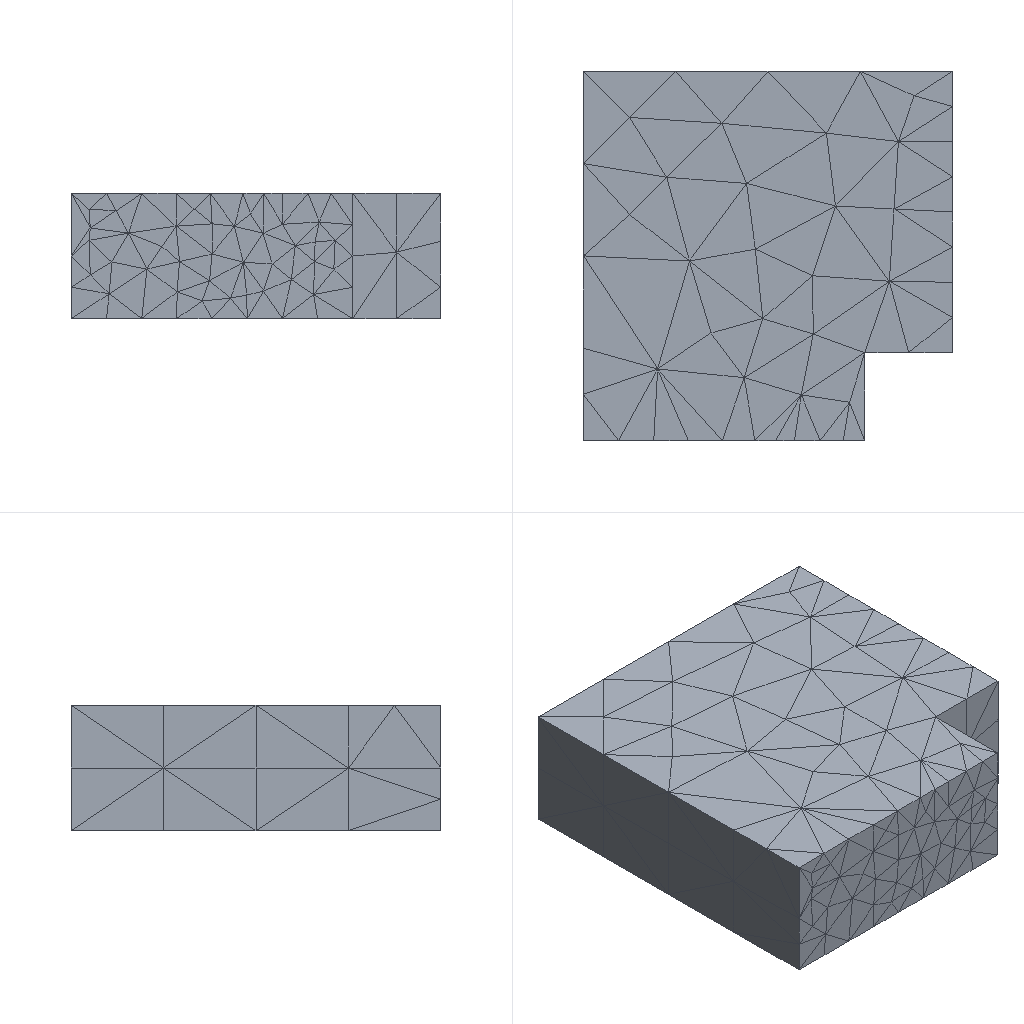Simulation study | ansys electronics desktop
Set-up summary:
category,name,step,type,value,unit,region
solver,ansys_electronics_desktop
units,length mm,,stated,model units
analysis,DESIGN_1,,HFSS Modal Network,design_type=HFSS
setup,Setup1,DESIGN_1,HfssDriven,frequency=10GHz; max_passes=6; max_delta_s=0.02
sweep,Sweep1,Setup1,Discrete,8GHz..12GHz n=9 step=
mesh,nodes,,,n/a (no mesh stored)
mesh,elements,,,n/a (no mesh stored)
material,vacuum,,permittivity,1
load,1,DESIGN_1,wave port,,,faces 9
load,2,DESIGN_1,wave port,,,faces 40
bc,PerfE,DESIGN_1,perfect e,,,"faces 7, 10, 11, 8, 12, 37"
Ansys Electronics Desktop project file, long lists of numbers shortened, first 464 of 1677 lines:
$begin 'AnsoftProject'
	Created='Fri Sep  4 17:11:43 2026'
	Product='ElectronicsDesktop'
	FileOwnedByWorkbench=false
	$begin 'Desktop'
		Version(2026, 1)
		InfrastructureVersion(1, 0)
		$begin 'FactoryHeader'
			$begin 'geometry3deditor'
				KernelVersion(2, 0)
				ProjectContainsGeometry3D='1'
			$end 'geometry3deditor'
		$end 'FactoryHeader'
	$end 'Desktop'
	UsesAdvancedFeatures=false
	PreviewImageDesignId=1
	NextUniqueID=0
	MoveBackwards=false
	$begin 'HFSSEnvironment'
		Version(1, 0)
	$end 'HFSSEnvironment'
	$begin 'PlanarEMEnvironment'
		Version(1, 0)
	$end 'PlanarEMEnvironment'
	$begin 'Q3DEnvironment'
		Version(1, 0)
	$end 'Q3DEnvironment'
	$begin '2DExtractorEnvironment'
		Version(1, 0)
	$end '2DExtractorEnvironment'
	$begin 'NexximEnvironment'
		Version(1, 0)
	$end 'NexximEnvironment'
	$begin 'NexximNetlistEnvironment'
		Version(1, 0)
	$end 'NexximNetlistEnvironment'
	$begin 'EmitEnvironment'
		Version(1, 0)
	$end 'EmitEnvironment'
	$begin 'Maxwell3DEnvironment'
		Version(1, 0)
	$end 'Maxwell3DEnvironment'
	$begin 'Maxwell2DEnvironment'
		Version(1, 0)
	$end 'Maxwell2DEnvironment'
	$begin 'RMxprtEnvironment'
		Version(1, 0)
	$end 'RMxprtEnvironment'
	$begin 'MaxCirEnvironment'
		Version(1, 0)
	$end 'MaxCirEnvironment'
	$begin 'SimplorerEnvironment'
		Version(1, 0)
	$end 'SimplorerEnvironment'
	$begin 'IcepakEnvironment'
		Version(1, 0)
	$end 'IcepakEnvironment'
	$begin 'IcepakFEAEnvironment'
		Version(1, 0)
	$end 'IcepakFEAEnvironment'
	$begin 'SchematicEnvironment'
		Version(1, 0)
	$end 'SchematicEnvironment'
	$begin 'geometry3deditor'
		Version(1, 0)
	$end 'geometry3deditor'
	ReadVersion=12
	$begin 'DesignMgrEnvironment'
		CompInstCounter=1
		GPortCounter=0
		NetCounter=0
		Alias('Ieee;Simplorer Elements\\Ieee', 'Std;Simplorer Elements\\Std', 'Basic_VHDLAMS;Simplorer Elements\\Basic Elements VHDLAMS\\Basic Elements VHDLAMS', 'Digital_Elements;Simplorer Elements\\Digital Elements\\Digital Elements', 'Transformations;Simplorer Elements\\Tools\\Transformations\\Transformations', 'HEV_VHDLAMS;Simplorer Elements\\HEV VHDLAMS\\HEV VHDLAMS', 'automotive_vda;Simplorer Elem
	$end 'DesignMgrEnvironment'
	$begin 'ProjectDatasets'
		NextUniqueID=0
		MoveBackwards=false
		DatasetType='ProjectDatasetType'
		$begin 'DatasetDefinitions'
		$end 'DatasetDefinitions'
	$end 'ProjectDatasets'
	VariableOrders[0:]
	$begin 'Definitions'
		$begin 'Materials'
			$begin 'vacuum'
				CoordinateSystemType='Cartesian'
				BulkOrSurfaceType=1
				$begin 'PhysicsTypes'
					set('Electromagnetic')
				$end 'PhysicsTypes'
				$begin 'AttachedData'
					$begin 'MatAppearanceData'
						property_data='appearance_data'
						Red=230
						Green=230
						Blue=230
						Transparency=0.95
					$end 'MatAppearanceData'
				$end 'AttachedData'
				permittivity='1'
				ModTime=1499970477
				Library='Materials'
				LibLocation='SysLibrary'
				ModSinceLib=false
			$end 'vacuum'
		$end 'Materials'
		$begin 'SurfaceMaterials'
			$begin 'Steel-oxidised-surface'
				CoordinateSystemType='Cartesian'
				BulkOrSurfaceType=2
				$begin 'PhysicsTypes'
					set('Thermal')
				$end 'PhysicsTypes'
				surface_emissivity='0.8'
				ModTime=1461288057
				Library='SurfaceMaterials'
				LibLocation='SysLibrary'
				ModSinceLib=false
			$end 'Steel-oxidised-surface'
		$end 'SurfaceMaterials'
		$begin 'Scripts'
		$end 'Scripts'
		$begin 'AnsysComponents'
			NextUniqueID=0
			MoveBackwards=false
			$begin 'AnsysComponentDefinitions'
			$end 'AnsysComponentDefinitions'
		$end 'AnsysComponents'
		$begin 'Symbols'
			$begin 'DESIGN_1'
				ModTime=1788513103
				Library=''
				ModSinceLib=false
				LibLocation='Project'
				HighestLevel=1
				Normalize=true
				InitialLevels(0, 1)
				$begin 'Graphics'
					Rect(0, 0, 0, 0, 0.00254, 0.00254, 0.00508, 0.00508, 0, 0, 0)
					Rect(0, 1, 0, 0, 0.0004233, 0.00254, 0.0004233, 0.0004233, 0, 0, 0)
				$end 'Graphics'
			$end 'DESIGN_1'
		$end 'Symbols'
		$begin 'DefInfo'
			DESIGN_1(1002, 0, 0, 0, '', 1788513103, '', 'DESIGN_1', '', '', '', '', '', 'Design.bmp', '', 'Project', '', '', 1788513103, '', 0, 0)
		$end 'DefInfo'
		$begin 'Compdefs'
			$begin 'DESIGN_1'
				Library=''
				CircuitEnv=0
				Refbase='U'
				NumParts=1
				ModSinceLib=true
				$begin 'Properties'
					TextProp('Representation', 'SRD', '', 'DESIGN_1')
					TextProp('Owner', 'SRD', '', 'HFSS')
				$end 'Properties'
				CompExtID=6
				$begin 'Parameters'
					ButtonProp('CosimDefinition', 'D', '', 'Edit', 'Edit', 40501, ButtonPropClientData())
					MenuProp('CoSimulator', 'D', '', 'DefaultNetlist', 0)
				$end 'Parameters'
				$begin 'CosimDefinitions'
					$begin 'CosimDefinition'
						CosimulatorType=4
						CosimDefName='DefaultNetlist'
						IsDefinition=true
						Connect=true
						Data()
						GRef()
					$end 'CosimDefinition'
					DefaultCosim='DefaultNetlist'
				$end 'CosimDefinitions'
			$end 'DESIGN_1'
		$end 'Compdefs'
	$end 'Definitions'
	DesignIDServer=2
	MoveBackwards=false
	$begin 'HFSSModel'
		RepRewriteV2=true
		Name='DESIGN_1'
		DesignID=0
		'Use Advanced DC Extrapolation'=false
		'Use Power S'=false
		'Export FRTM After Simulation'=false
		'Export Rays After Simulation'=false
		'Export After Simulation'=false
		'Allow Material Override'=false
		'Calculate Lossy Dielectrics'=false
		'Perform Minimal validation'=false
		$begin 'TemperatureSettings'
			IncludeTemperatureDependence=false
			EnableFeedback=false
			Temperatures(6, '22cel')
		$end 'TemperatureSettings'
		ObjsEnabledForDeformation()
		'Port Validation Settings'='Standard'
		'Save Adaptive support files'=false
		SolutionType='HFSS Modal Network'
		$begin 'DrivenOptions'
			AutoOpen=false
		$end 'DrivenOptions'
		HasTransientSetups=false
		MaterialDensity=1
		MassOfTissue=1
		VoxelSize=1
		TissueObjectList=-1
		AverageSarMethod=0
		UseAutoDCThickness=true
		HaveZwaveSupport=true
		SolveInsideThreshold=100000
		RequireBodyFaceInfo=false
		$begin 'OutputVariable'
			NextUniqueID=0
			MoveBackwards=false
		$end 'OutputVariable'
		$begin 'ModelSetup'
			$begin 'DesignDatasets'
				NextUniqueID=0
				MoveBackwards=false
				DatasetType='DesignDatasetType'
				$begin 'DatasetDefinitions'
				$end 'DatasetDefinitions'
			$end 'DesignDatasets'
			VariableOrders[0:]
			$begin 'Editor3D Doc Preferences'
				BackgroundColorVersion=1
				'Plane Background'=0
				'Need Lights'=true
				'Ambient Light'=8355711
				'Num Lights'=1
				Light0[4: 16777215, 0.75, -0.15, -0.63]
				Ver=2
			$end 'Editor3D Doc Preferences'
			SnapMode=31
			WorkingCS=1
			$begin 'GeometryCore'
				BlockVersionID=3
				DataVersion=2
				NativeKernel='PARASOLID'
				NativeKernelVersionID=26
				Units='mm'
				ModelExtents=10000
				InstanceID=-1
				$begin 'ValidationOptions'
					EntityCheckLevel='Strict'
					IgnoreUnclassifiedObjects=false
					SkipIntersectionChecks=false
				$end 'ValidationOptions'
				ContainsGeomLinkUDM=false
				$begin 'GeometryOperations'
					BlockVersionID=2
					$begin 'AnsoftRangedIDServerManager'
						$begin 'AnsoftRangedIDServer'
							IDServerObjectTypeID=0
							IDServerRangeMin=0
							IDServerRangeMax=2146483647
							NextUniqueID=68
							MoveBackwards=false
						$end 'AnsoftRangedIDServer'
						$begin 'AnsoftRangedIDServer'
							IDServerObjectTypeID=1
							IDServerRangeMin=2146483648
							IDServerRangeMax=2146485547
							NextUniqueID=2146483654
							MoveBackwards=false
						$end 'AnsoftRangedIDServer'
					$end 'AnsoftRangedIDServerManager'
					StartBackGroundFaceID=2146483648
					$begin 'CoordinateSystems'
					$end 'CoordinateSystems'
					$begin 'OperandCSs'
					$end 'OperandCSs'
					$begin 'SubModelDefinitions'
					$end 'SubModelDefinitions'
					$begin 'Groups'
					$end 'Groups'
					$begin 'UserDefinedModels'
					$end 'UserDefinedModels'
					$begin 'OperandUserDefinedModels'
					$end 'OperandUserDefinedModels'
					$begin 'ToplevelParts'
						$begin 'GeometryPart'
							$begin 'Attributes'
								Name='Arm1'
								Flags=''
								Color='(230 230 230)'
								Transparency=0.8
								PartCoordinateSystem=1
								UDMId=-1
								GroupId=-1
								MaterialValue='"vacuum"'
								SurfaceMaterialValue='""'
								SolveInside=true
								ShellElement=false
								ShellElementThickness='0mm'
								ReferenceTemperature='20cel'
								IsMaterialEditable=true
								IsSurfaceMaterialEditable=true
								UseMaterialAppearance=false
								IsLightweight=false
								IsAlwaysHidden=false
							$end 'Attributes'
							$begin 'PhysicsAttributes'
								SuppressedForPhysics='False'
								SuppressedForPhysicsEditable=true
							$end 'PhysicsAttributes'
							$begin 'Operations'
								$begin 'Operation'
									OperationType='Box'
									ID=5
									ReferenceCoordSystemID=1
									$begin 'BoxParameters'
										KernelVersion=24
										XPosition='0mm'
										YPosition='0mm'
										ZPosition='0mm'
										XSize='22.86mm'
										YSize='30mm'
										ZSize='10.16mm'
									$end 'BoxParameters'
									ParentPartID=6
									ReferenceUDMID=-1
									IsSuppressed=false
									$begin 'OperationIdentity'
										$begin 'Topology'
											NumLumps=1
											NumShells=1
											NumFaces=6
											NumWires=0
											NumLoops=6
											NumCoedges=24
											NumEdges=12
											NumVertices=8
										$end 'Topology'
										BodyID=6
										StartFaceID=7
										StartEdgeID=13
										StartVertexID=25
										NumNewFaces=6
										NumNewEdges=12
										NumNewVertices=8
										FaceNameAndIDMap()
										EdgeNameAndIDMap()
										VertexNameAndIDMap()
									$end 'OperationIdentity'
								$end 'Operation'
								$begin 'Operation'
									OperationType='Unite'
									ID=61
									$begin 'UniteParameters'
										KernelVersion=24
										KeepOriginals=false
										TurnOnNBodyBoolean=true
										BlankPart=6
										NumToolParts=1
										ToolParts(34)
									$end 'UniteParameters'
									ParentPartID=6
									ReferenceUDMID=-1
									IsSuppressed=false
									$begin 'OperationIdentity'
										$begin 'Topology'
											NumLumps=1
											NumShells=1
											NumFaces=8
											NumWires=0
											NumLoops=8
											NumCoedges=36
											NumEdges=18
											NumVertices=12
										$end 'Topology'
										BodyID=-1
										StartFaceID=-1
										StartEdgeID=62
										StartVertexID=63
										NumNewFaces=0
										NumNewEdges=1
										NumNewVertices=2
										FaceNameAndIDMap()
										EdgeNameAndIDMap()
										VertexNameAndIDMap()
										$begin 'GeomTopolBasedOperationIdentityHelper'
											$begin 'NewFaces'
											$end 'NewFaces'
											$begin 'NewEdges'
												$begin 'Edge'
													NormalizedSerialNum=0
													ID=62
													EdgeFaces(12, 37)
													$begin 'EdTolVts'
														TolVt(22.86, 7.14, 10.16, 5e-07)
														TolVt(22.86, 7.14, 0, 5e-07)
													$end 'EdTolVts'
													EdgeMidPoint(22.86, 7.14, 5.08)
												$end 'Edge'
											$end 'NewEdges'
											$begin 'NewVertices'
												$begin 'Vertex'
													NormalizedSerialNum=0
													ID=63
													VtPos(22.86, 7.14, 10.16)
												$end 'Vertex'
												$begin 'Vertex'
													NormalizedSerialNum=1
													ID=64
													VtPos(22.86, 7.14, 0)
												$end 'Vertex'
											$end 'NewVertices'
										$end 'GeomTopolBasedOperationIdentityHelper'
										$begin 'MergedFaces'
										$end 'MergedFaces'
										$begin 'MergedEdges'
										$end 'MergedEdges'
									$end 'OperationIdentity'
									BlankOperation=5
									NumToolOperations=1
									ToolOperations(33)
								$end 'Operation'
							$end 'Operations'
							$begin 'SubregionDependencyInformation'
								ChildSubregions[0:]
							$end 'SubregionDependencyInformation'
						$end 'GeometryPart'
					$end 'ToplevelParts'
					$begin 'OperandParts'
						$begin 'GeometryPart'
							$begin 'Attributes'
								Name='Arm2'
								Flags=''
								Color='(230 230 230)'
								Transparency=0.8
								PartCoordinateSystem=1
								UDMId=-1
								GroupId=-1
								MaterialValue='""'
								SurfaceMaterialValue='""'
								SolveInside=true
								ShellElement=false
								ShellElementThickness='0mm'
								ReferenceTemperature='20cel'
								IsMaterialEditable=true
								IsSurfaceMaterialEditable=true
								UseMaterialAppearance=false
								IsLightweight=false
								IsAlwaysHidden=false
							$end 'Attributes'
							$begin 'PhysicsAttributes'
								SuppressedForPhysics='False'
								SuppressedForPhysicsEditable=true
							$end 'PhysicsAttributes'
							$begin 'Operations'
								$begin 'Operation'
									OperationType='Box'
									ID=33
									ReferenceCoordSystemID=1
									$begin 'BoxParameters'
										KernelVersion=24
										XPosition='0mm'
										YPosition='7.14mm'
										ZPosition='0mm'
										XSize='30mm'
										YSize='22.86mm'
										ZSize='10.16mm'
									$end 'BoxParameters'
Last 344 lines:
								Increment=0.08727
								CreateIndexedSubsweepFlag=false
							$end 'PostprocessSweep'
							$begin 'PostprocessSweep'
								Variable='Theta'
								RegularSweep=1
								Units='deg'
								Minimum=0
								Maximum=6.283
								Increment=0.08727
								CreateIndexedSubsweepFlag=false
							$end 'PostprocessSweep'
							$begin 'PostprocessSweep'
								Variable='Phase'
								RegularSweep=1
								Units='deg'
								Minimum=0
								Maximum=6.283
								Increment=0.08727
								CreateIndexedSubsweepFlag=false
							$end 'PostprocessSweep'
						$end 'Sweeps'
						IsPortOnly=false
					$end 'SimDataExtractor'
				$end 'Solution'
				$begin 'Solution'
					ID=18
					Name='Sweep1'
					$begin 'SimDataExtractor'
						IsPortOnly=false
					$end 'SimDataExtractor'
				$end 'Solution'
			$end 'SimSetup'
			$begin 'Version ID Map'
				V=5
				$begin 'Setup'
					N='Setup1'
					V=0
					Soln(N='AdaptivePass', V=0)
					Soln(N='LastAdaptive', V=16)
					Soln(N='Sweep1', V=0)
				$end 'Setup'
				IQM=0
			$end 'Version ID Map'
			$begin 'ID Map'
				$begin 'Setup'
					N='Setup1'
					I=10
					Soln(N='AdaptivePass', I=11)
					Soln(N='LastAdaptive', I=12)
					Soln(N='Sweep1', I=18)
				$end 'Setup'
			$end 'ID Map'
			ValidationCacheHeader=''
		$end 'SolutionManager'
		$begin 'UserDefinedSolutionMgr'
			NextUniqueID=1000000
			MoveBackwards=false
		$end 'UserDefinedSolutionMgr'
		$begin 'DatasetSolutionMgr'
			NextUniqueID=2000000
			MoveBackwards=false
		$end 'DatasetSolutionMgr'
		Notes=$begin_cdata$ $end_cdata$
		$begin 'AnimationSetups'
		$end 'AnimationSetups'
		CacheHeaderFile='HDR6F9624520178851312848.tmp'
	$end 'HFSSModel'
	$begin 'DataInstances'
		DesignEditor='TopLevel'
		Refdes('0', 'U1')
		$begin 'CompInstances'
			$begin 'Compinst'
				ID='0'
				Status='Status'
				CompName='DESIGN_1'
				GatesInUse()
				$begin 'Properties'
					TextProp('ID', 'SRID', '', '0')
				$end 'Properties'
				$begin 'Parameters'
					MenuProp('CoSimulator', 'OHD', '', 'DefaultNetlist', 0)
					ButtonProp('CosimDefinition', 'OHD', '', 'Edit', 'Edit', 40501, ButtonPropClientData())
				$end 'Parameters'
			$end 'Compinst'
		$end 'CompInstances'
		$begin 'Instance'
			DesignEditor='DESIGN_1'
			ID='0'
			$begin 'HfssDesignInstance'
				DesignInstanceID=1
				$begin 'WindowPosition'
					$begin 'EditorWindow'
						Circuit(Editor3d(View('View Orientation Gadget'=1, WindowPos(3, -1, -1, -8, -31, 52, 52, 1657, 515), OrientationMatrix(0.03882, -0.02241, 0.03169, 0, 0.03882, 0.02241, -0.03169, 0, 0, 0.04482, 0.03169, 0, -1.164, -0.2277, -6.073, 1, 0, -2.542, 2.542, 
					$end 'EditorWindow'
				$end 'WindowPosition'
				$begin 'ReportSetup'
					$begin 'ReportManager'
						$begin 'Reports'
						$end 'Reports'
						NextUniqueID=0
						MoveBackwards=false
						$begin 'NextVersID'
							NextUniqueID=0
							MoveBackwards=false
						$end 'NextVersID'
					$end 'ReportManager'
					$begin 'Reports'
					$end 'Reports'
					$begin 'ReportsWindowInfoList'
					$end 'ReportsWindowInfoList'
				$end 'ReportSetup'
				$begin 'Properties'
				$end 'Properties'
				$begin 'UserDefinedDocument'
					$begin 'Data'
					$end 'Data'
				$end 'UserDefinedDocument'
			$end 'HfssDesignInstance'
		$end 'Instance'
		$begin 'SODInfo'
			$begin 'DESIGN_1'
				$begin 'CosimDefinition'
					CosimDefName='DefaultNetlist'
					$begin 'SODInstanceMap'
					$end 'SODInstanceMap'
					SODComponentList()
				$end 'CosimDefinition'
			$end 'DESIGN_1'
		$end 'SODInfo'
	$end 'DataInstances'
	$begin 'WBSystemIDToDesignInstanceIDMap'
	$end 'WBSystemIDToDesignInstanceIDMap'
	$begin 'WBSysIDSysDetails'
	$end 'WBSysIDSysDetails'
	$begin 'WBConnIDConnDetails'
	$end 'WBConnIDConnDetails'
	$begin 'WBMaterialGuidDetails'
		WBMaterialGuidMap()
	$end 'WBMaterialGuidDetails'
	$begin 'MinervaProjectSettingsBlk'
		MinervaRemoteFilePath=''
		FolderContainerString=''
	$end 'MinervaProjectSettingsBlk'
$end 'AnsoftProject'
$begin 'AllReferencedFilesForProject'
$end 'AllReferencedFilesForProject'
$begin 'ProjectPreview'
	ProductName='ElectronicsDesktop'
	MajorVersion=2026
	MinorVersion=1
	IsEncrypted=false
	Thumbnail64='/9j/4AAQSkZJRgABAQAAAQABAAD/2wBDAAEBAQEBAQEBAQEBAQEBAQEBAQEBAQEBAQEBAQEBAQEBAQE\
BAQICAQECAQEBAgICAgICAgICAQICAgICAgICAgL/2wBDAQEBAQEBAQEBAQECAQEBAgICAgICAgICAg\
ICAgICAgICAgICAgICAgICAgICAgICAgICAgICAgICAgICAgICAgL/wAARCABgAGADASIAAhEBAxEB/\
8QAHwAAAQUBAQEBAQEAAAAAAAAAAAECAwQFBgcICQoL/8QAtRAAAgEDAwIEAwUFBAQAAAF9AQIDAAQR\
BRIhMUEGE1FhByJxFDKBkaEII0KxwRVS0fAkM2JyggkKFhcYGRolJicoKSo0NTY3ODk6Q0RFRkdISUp\
TVFVWV1hZWmNkZWZnaGlqc3R1dnd4eXqDhIWGh4iJipKTlJWWl5iZmqKjpKWmp6ipqrKztLW2t7i5us\
LDxMXGx8jJytLT1NXW19jZ2uHi4+Tl5ufo6erx8vP09fb3+Pn6/8QAHwEAAwEBAQEBAQEBAQAAAAAAA\
AECAwQFBgcICQoL/8QAtREAAgECBAQDBAcFBAQAAQJ3AAECAxEEBSExBhJBUQdhcRMiMoEIFEKRobHB\
CSMzUvAVYnLRChYkNOEl8RcYGRomJygpKjU2Nzg5OkNERUZHSElKU1RVVldYWVpjZGVmZ2hpanN0dXZ\
3eHl6goOEhYaHiImKkpOUlZaXmJmaoqOkpaanqKmqsrO0tba3uLm6wsPExcbHyMnK0tPU1dbX2Nna4u\
Pk5ebn6Onq8vP09fb3+Pn6/9oADAMBAAIRAxEAPwD+rnTfH/7fXxx/aA/bO8I/BT43fsgfB/4Zfsz/A\
LQHgn4F+GdH+KX7HPxo+OvjvxF/bf7IH7LP7SGs+Kdd8b+E/wBvL4e6fHu8QftB6rp1rY2/hyP7PZ+H\
Ld5by6nmkZfQP+Fc/wDBU3/o8j9gD/xWn+0V/wDTYq/Er/goPrX7Z3hTV/2tvHv7EOj/ALQnif4g/C7\
/AILq/Ar4wfEHwV+zvbfETUNY+I3wl+D/APwQr/Zp+J+q/C34h6P8Oo3l8RfDLxT448J+APDtxpWpRz\
aZqur+JtG05oZr+6sIn8I+Cn7Qv/BZf9k74Jfs6eDPFp/aP8YRfDf9nj/gpV4n+OPxJ/ap+HWu6n4Iu\
/G3w21f/gqj4z+BHjX42/tL/Fbw1d3nh3RftvwR/ZEi02bV/FvgvQ7Hwn8RdINpB41sPFtnc+AwD+iz\
/hXP/BU3/o8j9gD/AMVp/tFf/TYqP+Fc/wDBU3/o8j9gD/xWn+0V/wDTYq8t/wCCVXx5+K3x18K/tbD\
4n/FL4s/F2y+FP7Vmi/DX4ZeKvjn8EvCX7PnxWT4f3v7GX7H/AMWbjT/GPwz8I/D7wwmk6gfiP8U/iH\
dq15pMN6YdViiZYbWG1tLb5v8A+Ca+k/GWy/bC/a98RfG34n/tOX2oz/Fz9vKPQ/hr8afgj/wVO8PfD\
nwx8L4f24/E5+COu+Bfj18ev2htR/Zp8Y+HG+CNn4Hk8Mad8Nvh1oHiCHwxrkMdtq81npPi6XWgD7i/\
4Vz/AMFTf+jyP2AP/Faf7RX/ANNio/4Vz/wVN/6PI/YA/wDFaf7RX/02Kv8APS+EuqftaXnhTwt+33q\
kX7SnxA+InwL8SfA+81r9oLxdffEz4weD4/FXww0jwPpPjeX4n/HXx/rmp3eneL7vxz4t+EzaR4eubx\
re60vxZrVtplva6RoKWcf7pfCj/gpF/wAFK/2M/gZ8F/2kvj14++NP7Q37PFpqPg3wl4b8D/GT4ceC/\
h1/wuzwh49+I/8AwVN+Gvgm40/9o+4+Ds/iLxH4h0n4Tfsm/sY/EFdYu7rXtV1/TvjlPqWv3Wo23i/Q\
NXtAD93P2sfFv/BU39l/9lj9pb9pf/hqD9gDxx/wzv8As/8Axk+On/CFf8O7v2ivDP8AwmH/AAqT4de\
I/H//AAi3/CR/8PS9Q/4R/wDtD/hH/sn277BffZPtfn/Y7ny/Jf8AX6v4pfjT/wAFLfi34D/4JRftIf\
Bbxf8AsxftDeNPgD+03pv/AAVT/Zp/Zz/au+L37Qmp/Ev4kSXPjT4tftXeDPhV8L/iloXxRvta8XWet\
eCdGudJ8H3z+J/FE+py2/wtvrjTm1O3tY9/70/tE/8ABUPxN4G/a31L9h/9lv8AZU8R/tZ/tC+FfBNn\
498faCvxe8C/A7w54Y0bUNM0XXLa1tvE3jmxuo9c1ddC8SeHruaFIoVWLW4FhluJVuktgD9caK/FH4q\
f8Fa/ip8Jf2PPG37T/jH/AIJ9/HTwL4p+E3xX8LfDz4rfCX4uaprHwzsNO8OeK5tS0iy+JXw4+Kdz8M\
b6w+K3hlfFkehaW32KytlEuupcPPHbNYyaj7j+2j/wUs0H9mP4ffsoeJ/hb8Mv+Gh/F/7Zfjrwb4W+C\
vgWDx0vw8Ou6H4y0bTdStPFi66nhDXjJBHe+J/A1qbdLI7z4rSU3CCHZKAfp7RX4r+L/wDgrR8SPFX7\
RHx8/Z7/AGMf2IPGH7XGpfswalNofxp8RJ8bvh/8GotI1uxv9U0jVrDwloPirSL688a/Ztb0TWLDFus\
VxNd6ZIkNs8MlrPcfpB+y18e9R/aS+D2h/E7W/gv8Yv2fvEF5d32leIPhZ8cfBGveBvGvh7V9NaIXBi\
tNe021bXfD00c8EtlqdvEILmOQo6QXcF1a24B+M/iP49fFf9nf9q/9u/UtM/a7/Zb/AGbfAXx6/wCCq\
37OH7L3w60X44/sRftB/tO+I/Gv7S3xN/4JefsC33hTRrXxv8Gv2v8AwJZeCPDWo6DoAjRta0NNO02f\
QLu71HxOsWoWlnZ7ngn9vHxR8bvg78PviXbf8Fgf+CPFv8K/2gPD/wAQ5/h/a/Gr9gP44fBnUPiV4U8\
C+KfF/wANviPcWnw0+O3/AAVg0HWtR8OWfiPwX4xsL2S40kWskWkTygy2bJM/xp+3V8K/hr+1J8Uf2+\
fgB4l+IP7Unwg8Z/DH/gqn8Kf2ofCHxF+B3/BOD9s/9t3w5a67Z/8ABFX9lf4L+C4LrX/2dfhzeaHoH\
iXS/F/xDtfEb6fda4mqiDwhaRTada2uvWOrReGX37IHgix+A3wC/Zw8C/tc/wDBRDw18Jf2fPHjfFTw\
x4A1X/ghH/wVv1r4ear8RbH9vHx9+2homueJvh5ong3RtK8b6b/YnjLRvBmoad4nt/ENsw8Bab4j0H/\
hG7ubUtPvgD9B/En7HvhPxd8KU0YeI/8AghH8d/hp+z9peueO9E+Fnwn/AOCFnjf9pq8+HGnfEzxx4h\
8CeJfEXw/+Bvwf/wCCjPiTVrSXxB8RPgn4v0q/k0LRHm1XVvg5q1rcCe58N3y2Pzf+2Z/wVL+Ntl+yX\
8adU8Fft2/srfF063ot/wDB++0X4d/8ErP23vgXrGneL/Gcn/CKeLfhs/xz+KP7bmt+Gvg/+0ToHhXU\
tY1258Ia9pd34v0600UXt34WS0dblfrn4GfF3wj+z3+xj4T/AGN/h/8AEH9sqPRPhT8I/h/8LfhL451\
X/ggd/wAFNdW1FbfwP438UXuow/GbwlqHwAl0f4p+EfEXwn/4V34V1+x0228KazcTWHi7xHZeJbDUvF\
Gjx+DPmL9lT4M/sn/szfG34Q/FS3f9s248OfB7xb8R/i3ovw++Gn/BFT/gtP8ACzQ9Q+M3xS8CfFf4X\
axqknhPUfDfiTwJonw10P4X/GHWfCnhDStM8BWfirR/CfgLwX4d1Lx5r2neGo47wA/P79mD/gndbfF3\
4V/CT9mzwr/wV2+KPgPVv2l/hT4M+KTfsuaD8Evj3efs9Xvif4ofA7Rf2lLH4Ya/8R9P+KNj4C1z4oy\
fB59J8T3OhToviWTw9Yr4gXQpdLiiuW+Mvi38cvjt8Qv+CTvhj4E/EX4hfD5PD37IP7ZnhH4VXHwWu/\
gp470T47+GL3xJ8Ov2itd8HeJvFfxp1T40TaPqXheGXSvir4ei8Mx/D7TdUsn8KWctxrnl2pt9R/oD+\
BXibxB8BZP2cdD0f46/tEePPhv+yf8Asj+AP2cfgT4S+JP/AAbp/wDBYvUtT8C+PvAv7Nlj8F7v45WO\
ueFL3RrG+1TXfGul2Wp6rZX2i3eq2vg651TwD4b8T+H213WvFN/yvi6DQbfwP+0T4p8MeIv2nvHv7TH\
xf+L37AHxasPE+uf8ENf+Cp/wH+HHi/W/2A/2oPDP7QvhXxZ8edG+F/7Kes/8Jb8cvFum6RLoPjDxho\
OneH7LULHw/wCHLbS/Ceh2ujpFIAfAX/BU3Xddn/4J9+Dvh34C8d/szX/7Nfwb/a40Lwv4Z8D/ALNf/\
BJ/9qj/AIJ7fDG38b634c/afn1bxD8HfiZ8Yf2hfE3gb42eBG8Q6B8SpNX/AOEB0zULafVPEVjrV14h\
t47y3j1z7w/4KyeD/wDgnV4l/bE1y+/aij/an/ZA+MWk6N4YuvCX7ZXwe0C58Z/CLx5Z6Z4N8NXehRe\
LLHw3YahrGm/ETTb2+1PSkt7HT7WZdP8ADunXl1rgt7q0tLX8wfif+3T8N/2cP2Fv+Cpnw/8AB3w+sf\
FVh8YPhP4F/Yti8f8Awh/Yy+JX7EPwN8Zyt8CPjtb/ABy+KPjj4XXvwz07Rfhd+2bbp441fSNZ0/Uof\
Dl14ksvBHhe60XwkPDvhLUlT9NfGH7Tn7Vnj7UP2gfjLZ6r8DPAerfAH9ob4ufA34/6/rMXjyXwFbXf\
wB03w5oK+MfAfghddF5b2OpQadpU00F54nR9P+2XDo2osCU+Q4x484X8PsJlOZcXYmpgMpzbHUMuWJp\
wjUjQr4mFWVCVWm5RnOFSdJYeMKPPWlWrUlTp1G+V/BeIXFuc8F5Tl+d5VwliOLcFDGQhmccLNRrYDL\
XQxM6uYwpck5Yr2Nenh6TwtNKtV+sfueepGNOfuH/BL7R/2kv24/2KP22v2f8A9p3xh4++Kv7P3iefW\
fhZ+yx8e/jB4W1LQPH3jvwvf6f4rtB42uYNckm1DVbLTdQs/h5rFjPe3GpTW2o3t7pp1K7GneVb/A3/\
AAR68P8Axh/ax/bP+AvhP466LPb+G/8Agkd8HPHHw9Gn3zyXcR+K+o/Efxn4d8IW2owugGn6rYaM0Fv\
bqhKj/hRtrMSWkaNXeMP+CmXxk+E//BPzw98U/wBnG6ufgT8V/iJouj32oeAdHsNP8S/Dv4eeD9E+Iu\
h6DrXxD8B/DzxrBdaN4A/tPXtT0mGNtOsEj1eL4w6jfaxp+r6vDpniPRPqrwR46X/gk98DfhzpvhHxx\
4Ri/aU/a/8A26Phf4b/AGnPjr+1lpEeu+C9Q8G/ETTfHCeM/jr4IPgn4ueHl1n4d+GPEtjLdXJ1vXNL\
1qxXxLPd+LdK8ODxJoRX7ScIWVTD4injcNNJxrUZqdOV+ZW5l8Mk4zjKEkpxlCUWrxZ7nDfFGS8V4Gt\
j8lxsMVTwuJxWDrxjKEpUMXgq0sPi8PU5JSiqlCtFwnyylG9mm1JN+Gf8FFvhx/wTk0D9sD4y+N/FHj\
L9uX/gnH+1FZaheeKdH+L3hf4danrvwl+OvirUkeY+L/hVN8NdY1HUZNR1G4W3muZ/7U8K25ub2Zb+K\
HVPtyxfth/wRl+Jn7W/xa/Yg8LeL/2x7bxC3xAm8X+I7HwRr3jHR/7C8ZeMPhPaWWhHwv4n8UWL2sEk\
1/Lq03iW3gvJoI5tR0/TLLUJGuWuvtlxi/s6/t8/G74naN+2M+l/DzwV+1sn7PXjz4R+Cfgt8Tf2V7O\
88GfDL9pW/wDilbaXb6xaaBc+NfiH4ostAtvB2s6nA3ivVYfEeq2Vlpqz3scUhtliufov/gmt+1F42/\
bP/Yq+Df7S3xF0Pwr4a8X/ABKm+Jranofgq31e18N6fb+EPi/4/wDAejRWMWu6vf3TTNofhfTXupJLl\
llu5Z5Yo7eF47eLI+hPzd+Mf7ef/Du/Vf8Agpt8av8AhVX/AAt//hKP+CrPwb+F3/CNf8Jz/wAK/wDs\
P9tf8Egf2D/Fn9u/2z/wh+t/afK/4Qn7P9l+yR7/AO0/N+0J5Ply/H3/ABFE/wDVjf8A5sx/+T9Xmf8\
AwWP/AOSP/wDBQv8A7TZfs/f+uUf2Sq/l/r+TfF/xM434W4zr5TkWd/Ucvhh8PNU/q2Eq2lOLcnz1sP\
Unq+nNZdEj/oM/Zy/Qf+i948fRpyzxA8V/DD/Wri7EZxm2Fni/7a4hwN6GGq040Kf1fLc2weFXJGTXM\
qKnK95yk7H+hl/wS7/4Kif8PJv+F5f8WN/4Ux/wpj/hWf8AzUz/AIWL/wAJJ/wsX/hYP/VPtC/sf7H/\
AMIJ/wBPX2j+1f8Alh5H770f/gr1e/tUaf8A8E0f2x5/2KPD3xA8T/tNyfCDUbL4aab8J9VuNH+KdsN\
S1bSNO8Z+Ifhpd6df22oTfEDSPh9deK9V0a10eRtevtR0W2svD9vd61cWFrN+KX/Brt/zfJ/3bP8A+/\
A1/Tv8ZfjN4L+A3ge8+InxAtPiJd+GNPuoLW+Pwx+Dfxg+OfiK0E8c8xv7jwT8EPAviLWotEhhtpnut\
QbTxY2aANd3EKuhb9x8LM8zTiPgPIs6zrFfXMyxn1r2tXkp0+b2eMxFKHuUoU6atTpwj7sFe13eTbf+\
WX09PC7gTwX+lh4reGnhpkX+rXBPDX9hfUsF9axmM9j9c4byfMMT/tOYYjFYup7TF4rEVv3uIqcntPZ\
0+WlGEI/yt+M9e/a/8RftKfCvxF8R/Cn/AAWH8AfB3W/jf+3Vqv8AwUP8B+Af+G4L+88FfDzVvHvjS+\
/4Jp+Gv2cb39mjX9b0K+n0zwtN4Es/G7/AnWNY0OR7G4fxdqV9ZvPdXHov/BPb4a/8FHfjN4HtvhV8a\
/iz+298EP2kvHP7JP7TXhb9sD4p/HTwt+0h4n+C3hL4r6l+0d8B4f2VtT/Z00n4ieJNG8Fv4qn/AGUh\
8aLTVp/hrqltNp+q3y6h4jkOvW0SS/tO/wDwVS/Yik8PWXjHRviJ8SvGngvWbnRNP8KeN/ht+y9+1X8\
UPA/xC1nXdB1LxRH4c+FvjP4d/BPVNM+K3iqy8N6J4hv9a0nw3d6pqXh608L6tca9a6dFpOota+j/AL\
PP7fv7Jn7Vni248F/AP4oXnj3V18Kar450q/Hw2+K/hfwf4x8I+Htb0Lwz4o1/4b/ELxn4G07QPihYa\
P4n8TaBpmtt4c1PVDouparDp+qraXjGEfoJ/IB+RH/BRz/gm/peif8ABGX9rP4PePNf+Dsfw9/Zm+CX\
xE/aW+EOi/s9/A3xb8FJl8V/Bf4Q/FHW/FEHxC1Px/8AtAfEOfx3qHifRLy5sJdVL2N9ZTXk+oXLau7\
xQQeRfFf/AIJtfEmx8R/E/wCG2s/HHw5rvhHXP2htW/ag+Jdv41+D93qngP48/Fb4m6PYeJdXi1PwV4\
P+N2i6loPgnSfETWz2+i3us6na3culWM1y1wltMtx+zf8AwVi/5RZf8FLP+zAP2yP/AFnX4jV8UftqX\
+pJ+0D8SrW58Q6rb6DIng6FtGSeQWTSv4K8LzLNAFMjwXC3AWQGNFVGjMoVZA01fzx9JTw+8XPEng7h\
rIfBerhcNxZh89wmKqV8XHDzjh8HTweYUp16UcTCrT+sQxNbC+xnGjUrUZP29D2dalCvS/G/Hf6SeT/\
Rg8O8y4vzfg2fGr4vnHh7C0KdX2M8Li8TTq5lSxiqWbUIxyqphqyScp4fE1YKFTm9nP8AKv8AaM/ZB0\
j46eG9Y8Iav4807RfHusaPpXhW58efDfRPHng/4bnw94S8aP4w0bSI/gU3xcudN1PTbVHvrK1e+v74p\
MU1GzljSCytrf7k8efs5eHv2idB/Ze+HuveMn0jRfg78fvhB8XL7TfGOmXnxIb4g6b8KdB1q1PgLxVe\
eLPE0dxeS6xHrtxZzarqc2q3UstxL51pqDzzGvHrzxPa2jSQaW5ZzKwknQi5up5IpFjd5FkysPJkDiQ\
gfMzKkb5A7vw18ZI/hidP8ReJ9Rl0a2tzLbCFLa91LxFdzX+lS6P9ntdJtoWv7ydUtb6WJ7SPKW1pPc\
n9zbedX9D/AEfvA7OfBbwXxmTeKfHOFxmOlGpOjVrVFhKEKko+0jhMJTqaKjRmnUpUsNRpUqEJVI/V6\
VOLa/ys+jJ9JnNqPiZnGN4zzSpw/wAG5pia2Jy7J4uWIVLFY+WFp16WFw9KEq9VOhgqHscOp1aGCjDE\
TpKm8RiqtX7c/Z5+DHjH9i34lfGXxX8FtSl8e/Az4ya1ovjPXf2c/EOua3b+IfBfj63tEh8d/En4ZfE\
3xb4g1OPxL4l8RQ2xa78Pa9HpNpqOq3NtdTeMtEtLN4bj6B/4Je/DPwN+zx+yH8OP2XvDXxQj+I3if4\
IR+Kk8c2ureH9N8CeP/Cuo/Eb4lePviBaaX43+HFl4y14+GJFfWdRttPvItUv9K8QWmjDXNC1C/wBIv\
bW5f8qZvjT8Tfi5fpP/AGrq/wAOvDivZ2b6ZZT2Fz4/vCiOLtZ/Glvd3SeGdMlF3dCFNHKavbvbwaja\
a/YTyyWFv+kH7AemWWk/FH43WdhE8cR+DP7NF7NJNcXF5eX2o6n4z/aj1PVtW1TUb2WS41bWb3VLy8u\
729uZZbq9u72a6uppbiaSRvZzHJ3gcJgcdTxUcXhcdzqElGULuDcZWUvespJq8owbauk42Z/rf4a+Kn\
CXixlFTPuDccsyydVKtOGIjfkqOhXrYaryNpXUa1CpC8eaMuW6k00fm5+2X4c8PeJ9M/4KT2HiXQdG8\
Q2MP/BXf4I3kVlrml2OrWkV3H/wRx/Yjhjuo7a/gkRLhYbidA4UMFndQcMwP5Sf8Ki+E/8A0TD4ef8A\
hFeG/wD5WV+03x48AeLviPe/8FM9D8GaT/bOqWv/AAVf+DWqz2v2/TNO8uwg/wCCP37CdnLP5+q3sEb\
YuL61XYrlz5uQpVWI+IP+GVvj1/0In/l0eDP/AJoq/wAIfp6cbZbkX0gsxwGJ4uoZNVjlWWT9hUx9PD\
ySlSm1L2cqsGlK10+XW25/vf8AQc8RMp4a8BsvyvGcdYfIK0MzzKf1ermdLCySnUg1P2Mq9NpStdS5f\
ete7P0b/wCCJfhDwn4V/wCGmf8AhF/DHh3w39v/AOFM/bv7B0XTdH+2/Zf+Fr/Zvtf9n20f2jy/tFx5\
e/ds899uNzZ/Uv8Aaw+B/i/9ob4Rah8L/CfjT4deFbfXb5rbxnofxk+Bmi/tF/B74neBdR0PXNC1/wC\
HXxM+F2p+LPD11q3h6c6xaalbzaV4i0S+t9W8L6a89ze6QdU0XVPhf/glL8KvHvwy/wCF9f8ACb6D/Y\
n9t/8ACrv7M/4mmjal9q/s3/hYv23/AJBGo3Hk7Pt9p/rNm7zfk3bW2/Sf/BRX4ry/B79mrXPEml/tG\
j9lrxff6xFovw++Keraz8OvBngA+Oz4f8R634f8I/FT4o/Fz9nL4o+G/hP4D1eXRJrNta1Twypm1SbS\
9D03UItZ1nTrS9/0g+hZmlHOfoz+GuZYfMY5rRxP9s8uIhWVeNTk4gzWm7VYympcjg4O0nyuLjo1Zf5\
5fTFznD8QfSO8Rc3wuawzuhi/7I5cVTrxxMKvs8hyuk7VoynGfI4Om7SfK4OGjjZflx8IP+CB2q/s0e\
Lfgj4+/Zw/ar8JeEfHn7NOu/EbxF8KfG3xD/ZkvfiJ4r+IWsfGfw/458OfEjVP2vdZ0P8AaH8NyftHa\
ppth8T/AIkx/Dya1/4REeCYfH2rxTR+Iv7Qunl+sv8AgnZ/wSt1P9gS++EmhR/H/TPin8Jf2b/gx+0B\
8Fv2evB6/By48C+NPDWiftRfGn4W/Hz4yaj8SPiE/wAWdatviLdSePvhPoS6HHY6B4cTStOu57W5Oqz\
bbofjN4W/4KnfF/xZ4s/Z60fxf/wV7+H3ww0XxjY6RpP7dsmqfDj9jP4RfEL9i34hXfwN8YfEfQPDvg\
r4S/E7QPFWr+G9H0r4neH/AAT8O/ilrnj4eIdEuPG3xl0PRPAl9oOrDU9E0b7T/wCCM37e37T/AO1j4\
7+Fdp+0B8eYfHHxD8bfs2/tK/ED9pr9mRPCXwf8OSfsc/Ej4XftCfBD4efs56f9m8E+BNO8UaFF8Rvg\
34z8eeKBbeMNT1Vr46IbzQVs9Oia3T+pT+ZT9R/+CsX/ACiy/wCCln/ZgH7ZH/rOvxGr8xf2/NWgg/a\
m+KkV5eW9jp9ong+S8nnuUt4fKT4YeFbq4N1LI6qlutp5jMGO0KpkbgDb+nX/AAVi/wCUWX/BSz/swD\
9sj/1nX4jV+Mf7e/gTV/H37cH7Qc0t3eSaVoF98NbOwtfs01zYWd2Pgv8ACq7ivIYY5PLTVUuvENwyX\
DRtOqy+WsojKxj9W8HZ0Y8WVY1VByq4SpGDqS5YRl7ahJybUZN2hGfLFK8pcqvC/PH+QvprcB47j7wi\
y/CYDD1cW+H85w+Z1adCNGVadKjl+Z4eSp/WK1ClFqWKjKU5zfJBSnGnVmo05eES/EWSHR4JfBOjTW0\
1/EyHxrrkJtDaw3kCsk/hfwzfWzTXd4kUdzE02qQ[REDACTED]/mJtzNfS6tf3N3q2tXCSR3Gs\
6rcPe6lJFNN9pmtoppPlsNON2XlWztVgsopJGMFvEDiu21rSodG0qDT4FZEtL5oNsgIkMg+1mZ5FI+W\
Rpt7MOAC2AAAAOMuZ7eytpLy9ubaxs4tnm3d7PFa2sXmSLEhknndVXMroo55Zgo5IFf58/Sp4s4kzvx\
SzLJ6mbYjHZfSSjh6K5kmq1SVoRpqdRqMrQUcPGc6cWlyqU3Kc/8H8RmmbVsbj+Hsjy+WVwxOInhJ4b\
CyrV8XjpRreyp08XiLyq4qcnGCeGoxoZf7ZOrhcBh51Z830z4Q1e60SGK7j0bUNZ0pLzfqEukKt5q2n\
xRQ28qXUehhVl1i0Ful2ZI7Iz6i0iwQ2mnXrzOYf16/wCCfet6X4i+JPxn1fR7tbywufgn+zHEsnlzQ\
TQXVl4w/aisNQ0++s7qNJtN1W11G2ura7tLiOK5tLq0mtrmKKeKSNfnH9mz9if4x+NbOTV/EEtl8KvA\
91qkPk6z4l8KeIG+Kmq22mvb2urx+Hfhn498N6afBKTfatQSw1vxJHcvHe+GfNfwVrWhahY6nP8Ar18\
IPgb8Ofgjor6b4J0SFdY1K00uDxf461O30+58e/EG70gXv2HU/HHiW1sYH1maBtS1FbG2VIdN0i2u/w\
CzdEsdN0qG2sYf7FeY0avC/DWUxpRpYjK6clNU6bpUU5yclGlTl79OEU0owlrCK5Xqj/dT6Dvhhxp4X\
eCGQZLx1k74fzyc8fUng5uDq0Y1s2zHEUfaRpynGm50K1KoqblzwjNQqRjUU4R/NTwj/wAlO/4Kl/8A\
aS34Vf8Arpn/AIJ5Vs1y+g3Ulp8SP+CpMkaozN/wUy+FCEOGIwf+CS3/AAT1YkbWHOVFH9t3f/PO3/7\
4k/8Ajtf8tP7VjC1a30uM4nBLl/sLJFq/+nFQ/wBHOEvG7gTgTJ4cP8QYjE08xp1KlVqlhpVYclVpx9\
5SSvZarofcH7LH/M9/9yx/7sNe6fFP4v8Awm+Bng69+Inxs+KHw7+D3w/025sbLUfHPxT8beGvh94Os\
LzU7lLPTbS98TeLdTtLK1ubi7kjigjknV5ZHCRhmIFfO/7I17Lef8LB81Y18v8A4RPb5YYZ3/8ACS5z\
uc/3RS/tyfDj4+/Ez4SaFpP7NHgn9nbxb8VtM8fafqNhrH7RPiPVPB9t8N/Duo+FfGPhHxj49+D/AIs\
0z4FfEUeGvjkvhfxRqmj6LfXfhi9062tfF+py6hDqFosui6r/ALMfs1KcqX0KPBaE/ij/AKx3+fFufP\
8AU+K4n4oyrjPPMdxLkk51MrzL2XsnUg6c37GjTw8+aDba/eUppa6qz6m1rP7e37DHhxvF6eIf20P2T\
tBf4fSaDF49TWf2i/g/pbeCJfFTxp4Xi8XrfeMUPhqTUnmhFgt75BvDKotxIWGfSPh5+0l+zr8XfF/i\
j4ffCj4+fBb4n+PfBFjp+qeNPBHw8+Kfgbxp4v8ACGmatFbTaVqPijw14b125vdAsbmG9s3t5ruGGOZ\
buJo2YSKT/Op8Mv8Agjb+1n8Dvit+zb8YfhN4H/ZC062/ZY8TfHbxD4M+AHij9qb9o7xZ8HfFGg/tEe\
GvHHhaH4Y6B/bv7LtzZfs4aB8PvD3jya1vNU8IeFprn49634T0rx78SrDQ/FUML2n1v/wSp/4Jm/tFf\
sM3nwE8IfFjXvgn4k8Bfstfs9/tS/BXwN8QfAHjPx5rfxL+NF7+1X+0T8Gf2g9V1r4o+EvE3ws0ey8E\
weE5/hXd6Ho4tfEHiaXUrXxA13J/ZBD2b/3SeCfb3/BWL/lFl/wUs/7MA/bI/wDWdfiNXwr8bvDNrrf\
7Xf7U81y8zE+O/hXZpDEDsCyfBP8AZ1jmmm2kNIqx3RbCtHt8kksQSB91f8FYv+UWX/BSz/swD9sj/w\
BZ1+I1drqP7E/w58VfGf4mfF34h674m8Z2PxC8Q6Frkfwua4h8P/D61/sP4f8Aw38CeT4pg0VY9R+JF\
vcw+Arv7Zper6hL4VvLHxE1le+Gbme3/tCf08pzOtlOKeLoScaqi0nGye8Zbu9k+Wza1SfXZ+RnuUUM\
9yzFZXibewxkJwldN+7OEoN2TV2lJtK6u1ut1+SHw7/ZP139peXVj8Oltf8AhHrjxvqeqyfFvUX1Rfh\
pZeC3vNZ0axXwLqun6K9l8XfF41S4ubu50zR7s6dbr4OuNG1rxH4R1a5tkuv2D/Z+/Y4+FnwIXTtbNn\
Y+OfiJYYmsPG+t+HPD9k/g+a70M6LrVl8MdMs7Jn8F6TeQXGoR3NzPeap4l1OymtrHxH4l1+HTdONt9\
bUV83HKMshm2Lz1YKm84xsYwq4lrmqyhBNRgpyu4R11jDljJ6yTep+f+HXgj4Y+Fc8RiuDeFcNgM3xy\
axOYSpwnjsQ5VKlSbqYjlTjzzqSc40Y0qckoJwapwUSiiivRP1c/F7S/+Sif8FSP+0mvwn/9dKf8E96\
oV5R8Xv8AkL/8FN/+0q/wc/8AXQX7B1fI1f8AOL+0y4P/ALZ+lHm2O/tH6tzZLk8eX2PP8NGor83tYb\
9raH+dn0lPpGf8Q08T8Vwv/qd/bXssFg63t/7Q+rX9tCT5fZfUa9uW1ub2jv2R+9H7Hf8AzUX/ALlH/\
wB2evSf2qPjD8SfgZ8KL34hfDL4XeD/AIn3+kXlxc+J2+JHxp0f4BfDP4feB9I8O+IPEviT4ifEH4j3\
/hTxDead4ftYdCgsIodI8O65fzal4ksPOtbPSE1TWNM+Lv8AgmB/zXD/ALpp/wC9Ar7g/aP/AGYPg9+\
1h4K0H4f/ABr07xzqPhvwx488NfEzQT8PfjJ8ZvgZ4i03xx4O+3P4X1yDxr8C/H/hvWmaxu7+S6gt31\
BrRb61tL/yDeWNlPb/AOtf7PbLv7J+iB4RZf7b6x9X/t/3+Xkvz8UZ1P4eaVrc1vid7X0vY/q/6P8Ax\
n/xEHwj4S4v/s3+yP7X+v8A+z+2+sez+r5njcL/ABvZUefn9jz/AMKPLzcvvcvM/wAy4v8Agrz4r8af\
GI/s4fCH9lI6l+0HJoH7FO74cfGb40TfB3/hFfiV+1p+zD+1x+174k+FfxN1TRfhB4rm8Fa94N+Dn7K\
V2JJYbHU/7Z1zx5baa0GjWtk+pXXa/wDBO3/gqlqX7fd98INdi/Z9tPhZ8Jv2kfgr+0B8a/2f/GJ+Ll\
x428Ya/pP7L3xq+FnwC+Mei/ErwA3wq0a3+HGpRePvivoraIbTXvEK6pptnNdXA0ycfY19r8Zf8En/A\
NgPx743m+K/iT4ETv8AG268FfC3wBe/tD6H8W/jh4S/aY1Hw98HfDuu+EPB82qftK+EviVY+PNU8VXH\
hDxBcaR4k1+48Qy67400rStH07xjqWvWWg6JBp/pv7PH7AP7Jv7KXi278a/AP4Y6j4D1abwvqvgrTdO\
b4nfFzxX4L8HeFfEOtaF4m8U6J8Nfhz418eal4e+FllrPibwz4f1LXB4b0vSm1vUdIgv9Va8u0E1f2e\
fshw//AAVi/wCUWX/BSz/swD9sj/1nX4jV9/18Af8ABWL/AJRZf8FLP+zAP2yP/WdfiNX3/QAUUUUAF\
FFFAH//2Q=='
	$begin 'DesignInfo'
		DesignName='DESIGN_1'
		Notes=''
		Factory='HFSS'
		IsSolved=true
		'Nominal Setups'[1: 'Setup1']
		'Nominal Setup Types'[1: '']
		'Optimetrics Setups'[0:]
		'Optimetrics Experiment Types'[0:]
		Image64=''
	$end 'DesignInfo'
$end 'ProjectPreview'
Results summary, first 71 of 122 lines:
result,designs[0].name,1.step,,DESIGN_1
result,designs[0].design_type,1.step,,HFSS
result,designs[0].solution_type,1.step,,HFSS Modal Network
result,designs[0].setups[0].name,Setup1,,Setup1
result,designs[0].setups[0].SetupType,Setup1,,HfssDriven
result,designs[0].setups[0].SolveType,Setup1,,Single
result,designs[0].setups[0].Frequency,Setup1,,10GHz
result,designs[0].setups[0].MaximumPasses,Setup1,,6
result,designs[0].setups[0].MaxDeltaS,Setup1,,0.02
result,designs[0].setups[0].IsEnabled,Setup1,,true
result,designs[0].setups[0].sweeps[0].name,Sweep1,,Sweep1
result,designs[0].setups[0].sweeps[0].RangeType,Sweep1,,LinearCount
result,designs[0].setups[0].sweeps[0].RangeStart,Sweep1,,8GHz
result,designs[0].setups[0].sweeps[0].RangeEnd,Sweep1,,12GHz
result,designs[0].setups[0].sweeps[0].RangeCount,Sweep1,,9
result,designs[0].setups[0].sweeps[0].Type,Sweep1,,Discrete
result,designs[0].setups[0].sweeps[0].IsEnabled,Sweep1,,true
result,designs[0].boundaries[0].name,PerfE,,PerfE
result,designs[0].boundaries[0].BoundType,PerfE,,Perfect E
result,designs[0].excitations[0].name,1,,1
result,designs[0].excitations[0].BoundType,1,,Wave Port
result,designs[0].excitations[0].WavePortType,1,,Modal
result,designs[0].excitations[0].NumModes,1,,1
result,designs[0].excitations[1].name,2,,2
result,designs[0].excitations[1].BoundType,2,,Wave Port
result,designs[0].excitations[1].WavePortType,2,,Modal
result,designs[0].excitations[1].NumModes,2,,1
result,designs[0].materials_assigned[0],1.step,,vacuum
result,designs[0].objects,1.step,,2
result,designs[0].model_units,1.step,,mm
result,designs[0].valid_solutions[0],1.step,,Setup1 : AdaptivePass
result,designs[0].valid_solutions[1],1.step,,Setup1 : LastAdaptive
result,designs[0].valid_solutions[2],1.step,,Setup1 : Sweep1
result,designs[0].sparams[0].freq_hz[1],1.step,,8e+09
result,designs[0].sparams[0].freq_hz[2],1.step,,8.5e+09
result,designs[0].sparams[0].freq_hz[3],1.step,,9e+09
result,designs[0].sparams[0].freq_hz[4],1.step,,9.5e+09
result,designs[0].sparams[0].freq_hz[5],1.step,,1e+10
result,designs[0].sparams[0].freq_hz[6],1.step,,1.05e+10
result,designs[0].sparams[0].freq_hz[7],1.step,,1.1e+10
result,designs[0].sparams[0].freq_hz[8],1.step,,1.15e+10
result,designs[0].sparams[0].freq_hz[9],1.step,,1.2e+10
result,designs[0].sparams[0].expr,1.step,,"dB(S(1,1))"
result,designs[0].sparams[0].min_db,1.step,,-8.947
result,designs[0].sparams[0].solution,1.step,,Setup1 : Sweep1
result,designs[0].sparams[0].value_db[1],1.step,,-0.6571
result,designs[0].sparams[0].value_db[2],1.step,,-0.3047
result,designs[0].sparams[0].value_db[3],1.step,,-0.2298
result,designs[0].sparams[0].value_db[4],1.step,,-0.2414
result,designs[0].sparams[0].value_db[5],1.step,,-0.3544
result,designs[0].sparams[0].value_db[6],1.step,,-0.8378
result,designs[0].sparams[0].value_db[7],1.step,,-4.897
result,designs[0].sparams[0].value_db[8],1.step,,-8.947
result,designs[0].sparams[0].value_db[9],1.step,,-4.404
result,designs[0].sparams[0].max_db,1.step,,-0.2298
result,designs[0].sparams[1].freq_hz[1],1.step,,8e+09
result,designs[0].sparams[1].freq_hz[2],1.step,,8.5e+09
result,designs[0].sparams[1].freq_hz[3],1.step,,9e+09
result,designs[0].sparams[1].freq_hz[4],1.step,,9.5e+09
result,designs[0].sparams[1].freq_hz[5],1.step,,1e+10
result,designs[0].sparams[1].freq_hz[6],1.step,,1.05e+10
result,designs[0].sparams[1].freq_hz[7],1.step,,1.1e+10
result,designs[0].sparams[1].freq_hz[8],1.step,,1.15e+10
result,designs[0].sparams[1].freq_hz[9],1.step,,1.2e+10
result,designs[0].sparams[1].expr,1.step,,"dB(S(1,2))"
result,designs[0].sparams[1].min_db,1.step,,-12.879
result,designs[0].sparams[1].solution,1.step,,Setup1 : Sweep1
result,designs[0].sparams[1].value_db[1],1.step,,-8.526
result,designs[0].sparams[1].value_db[2],1.step,,-11.691
result,designs[0].sparams[1].value_db[3],1.step,,-12.879
result,designs[0].sparams[1].value_db[4],1.step,,-12.671